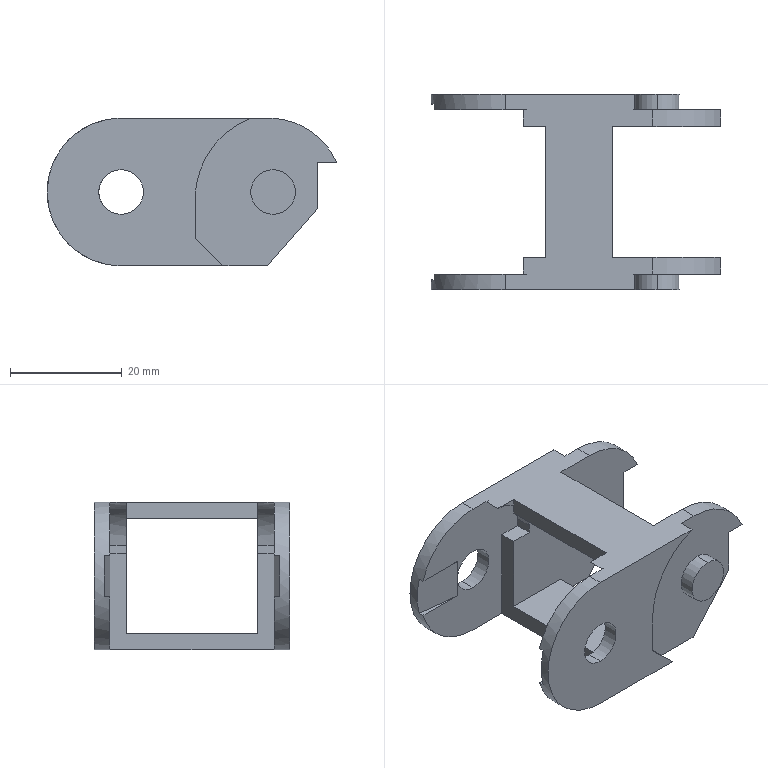Part | NX | features BREP 1 | 1 solid | 58 faces | box 51.916 x 35 x 26.5 mm | volume 9407 mm3 | plane 42 | cylinder 16 | commonest cylinder face diameters 8 x8 26.5 x4 17 x2 31.319 x2